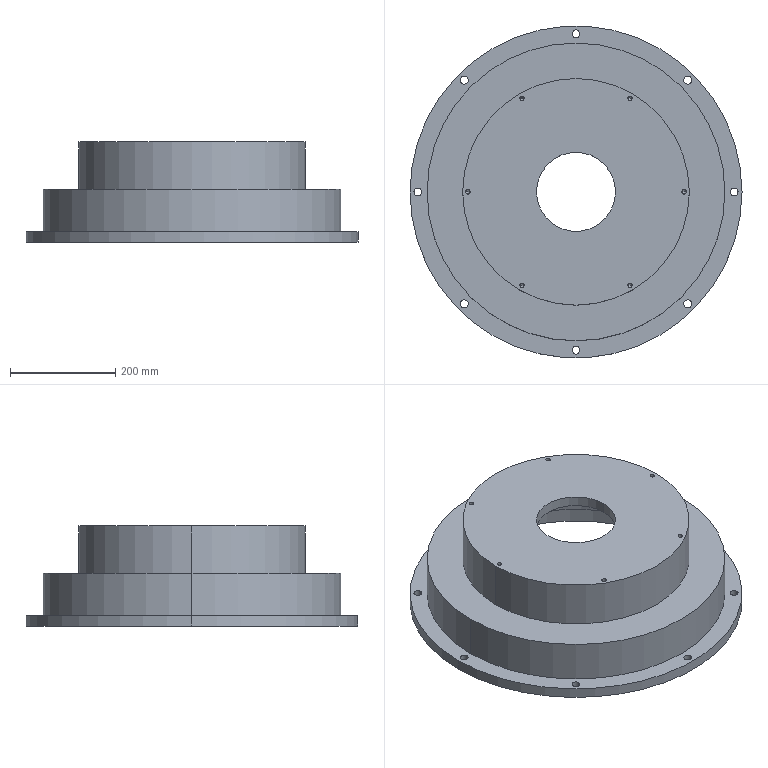Part | SolidWorks | features ICE 5, Extrusion 1, HoleWzd 1 | 1 solid | 58 faces | box 630 x 630 x 190 mm | volume 10873138 mm3 | cylinder 40 | cone 12 | plane 6 | commonest cylinder face diameters 15 x16 8.5 x12 150 x2 390 x2 430 x2 530 x2